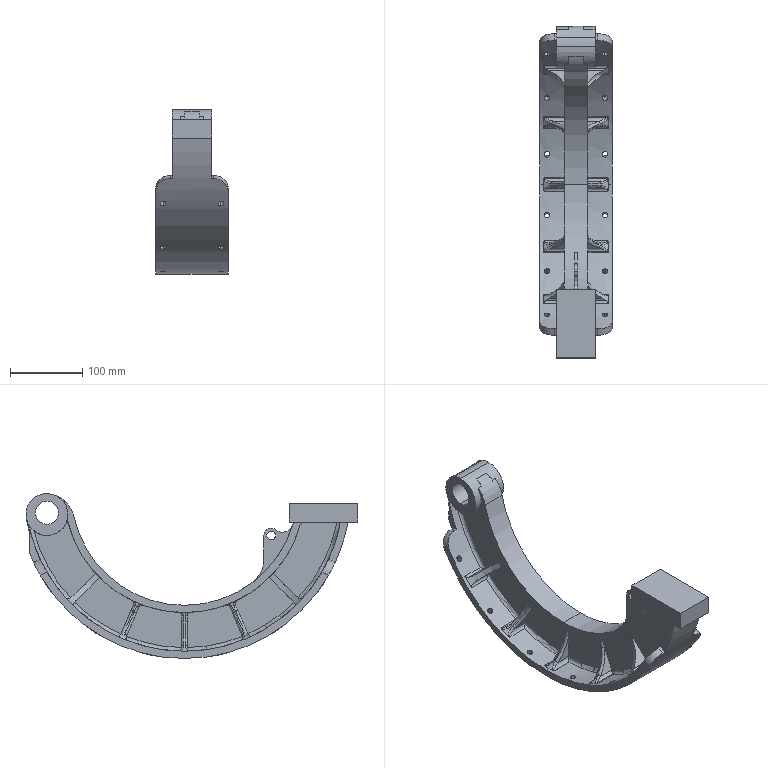Part | SolidWorks | features Cut 5, Boss 4, Fillet 4, CirPattern 3, MirrorPattern 2, RefAxis 1, RevCut 1, Revolution 1, Rib 1 | 1 solid | 257 faces | box 100 x 459 x 228 mm | volume 1537411 mm3 | cylinder 101 | plane 81 | torus 38 | spline 37 | commonest cylinder face diameters 10 x36 8 x24 118.94 x10 333 x6 40 x4 58 x4